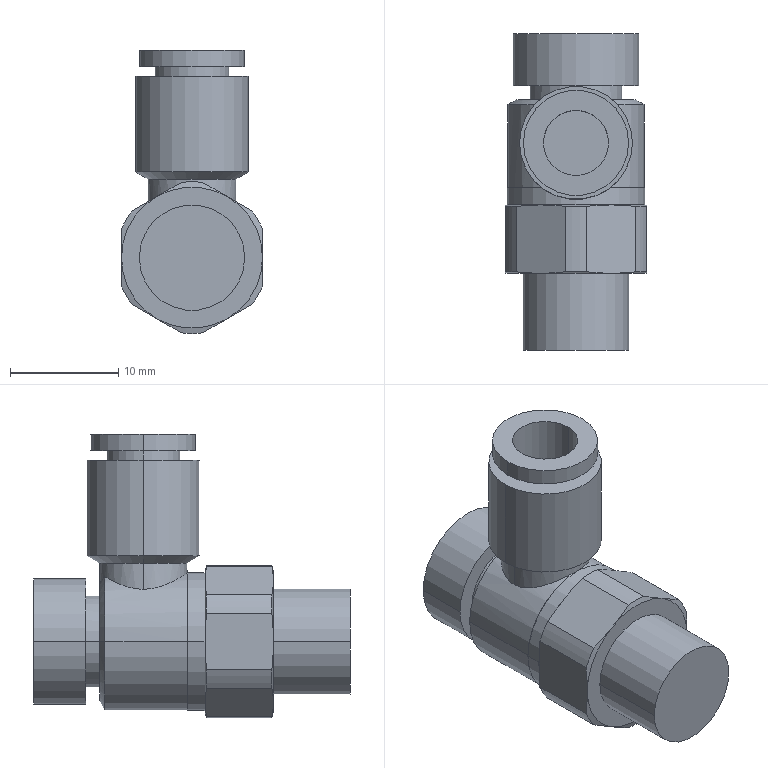Part | SolidWorks | features BaseBody 1 | 1 solid | 61 faces | box 13 x 29.2 x 26.1 mm | volume 3843 mm3 | cylinder 27 | cone 17 | plane 17 | commonest cylinder face diameters 14 x7 6 x2 6.79 x2 8.1 x2 8.45 x2 9.7 x2